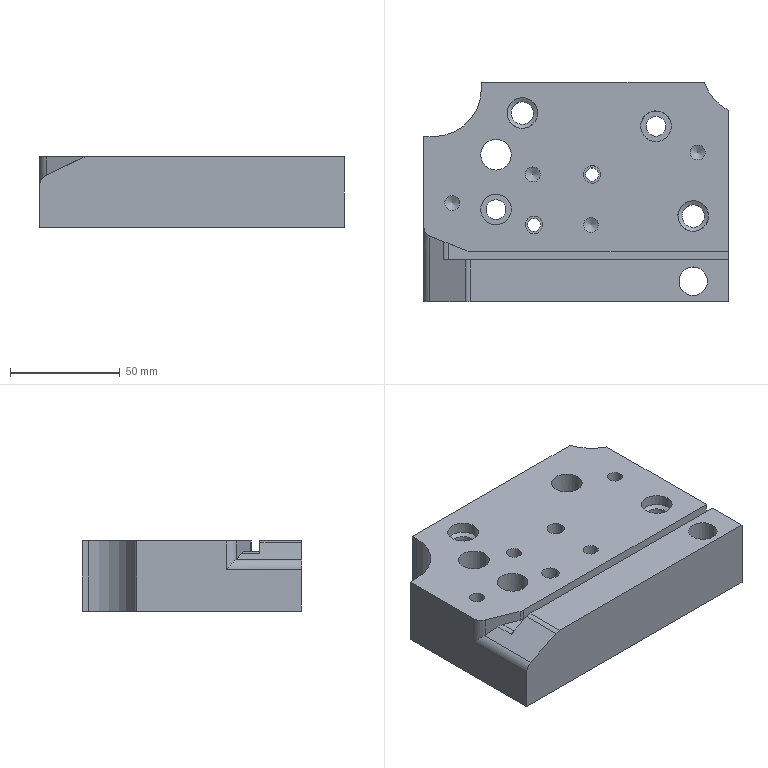Part | STEP file | gslz 2016.10.28-13_id1122_x_t | 1 solid | 57 faces | box 139 x 100 x 32 mm | volume 383578 mm3 | cylinder 29 | plane 20 | cone 8 | commonest cylinder face diameters 6.8 x6 10 x5 14 x5 6 x2 8 x2 9 x2